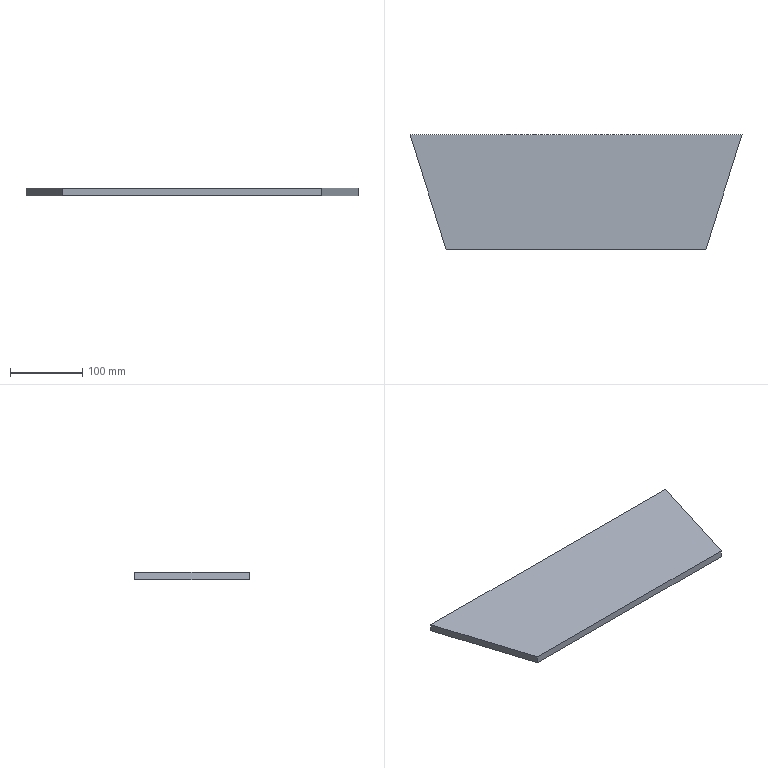Part | STEP file | 04-Vertical plate | 1 solid | 6 faces | box 460 x 159 x 10 mm | volume 651900 mm3 | plane 6
STEP:
#1=CARTESIAN_POINT('',(0.,0.,0.));
#2=DIRECTION('',(0.,0.,1.));
#3=DIRECTION('',(1.,0.,0.));
#4=AXIS2_PLACEMENT_3D('',#1,#2,#3);
#5=CARTESIAN_POINT('',(460.,0.,0.));
#6=VERTEX_POINT('',#5);
#7=CARTESIAN_POINT('',(0.,0.,0.));
#8=VERTEX_POINT('',#7);
#9=CARTESIAN_POINT('',(0.,0.,0.));
#10=DIRECTION('',(-1.,0.,0.));
#11=VECTOR('',#10,1.);
#12=LINE('',#9,#11);
#13=CARTESIAN_POINT('',(0.,0.,10.));
#14=DIRECTION('',(0.,-1.,0.));
#15=DIRECTION('',(0.,0.,-1.));
#16=AXIS2_PLACEMENT_3D('',#13,#14,#15);
#17=PLANE('',#16);
#18=CARTESIAN_POINT('',(10.,0.));
#19=DIRECTION('',(0.,-1.));
#20=VECTOR('',#19,1.);
#21=LINE('',#18,#20);
#22=(GEOMETRIC_REPRESENTATION_CONTEXT(2)PARAMETRIC_REPRESENTATION_CONTEXT()REPRESENTATION_CONTEXT('',''));
#23=DEFINITIONAL_REPRESENTATION('',(#21),#22);
#24=PCURVE('',#17,#23);
#25=CARTESIAN_POINT('',(0.,0.,0.));
#26=DIRECTION('',(0.,0.,-1.));
#27=DIRECTION('',(-1.,0.,0.));
#28=AXIS2_PLACEMENT_3D('',#25,#26,#27);
#29=PLANE('',#28);
#30=CARTESIAN_POINT('',(0.,0.));
#31=DIRECTION('',(1.,0.));
#32=VECTOR('',#31,1.);
#33=LINE('',#30,#32);
#34=(GEOMETRIC_REPRESENTATION_CONTEXT(2)PARAMETRIC_REPRESENTATION_CONTEXT()REPRESENTATION_CONTEXT('',''));
#35=DEFINITIONAL_REPRESENTATION('',(#33),#34);
#36=PCURVE('',#29,#35);
#37=SURFACE_CURVE('',#12,(#24,#36),.PCURVE_S1.);
#38=EDGE_CURVE('',#6,#8,#37,.T.);
#39=ORIENTED_EDGE('',*,*,#38,.T.);
#40=CARTESIAN_POINT('',(0.,0.,10.));
#41=VERTEX_POINT('',#40);
#42=CARTESIAN_POINT('',(0.,0.,10.));
#43=DIRECTION('',(0.,0.,-1.));
#44=VECTOR('',#43,1.);
#45=LINE('',#42,#44);
#46=CARTESIAN_POINT('',(0.,0.));
#47=DIRECTION('',(1.,0.));
#48=VECTOR('',#47,1.);
#49=LINE('',#46,#48);
#50=(GEOMETRIC_REPRESENTATION_CONTEXT(2)PARAMETRIC_REPRESENTATION_CONTEXT()REPRESENTATION_CONTEXT('',''));
#51=DEFINITIONAL_REPRESENTATION('',(#49),#50);
#52=PCURVE('',#17,#51);
#53=CARTESIAN_POINT('',(0.,0.,10.));
#54=DIRECTION('',(0.9539,0.3,0.));
#55=DIRECTION('',(-0.3,0.9539,0.));
#56=AXIS2_PLACEMENT_3D('',#53,#54,#55);
#57=PLANE('',#56);
#58=CARTESIAN_POINT('',(0.,0.));
#59=DIRECTION('',(0.,-1.));
#60=VECTOR('',#59,1.);
#61=LINE('',#58,#60);
#62=(GEOMETRIC_REPRESENTATION_CONTEXT(2)PARAMETRIC_REPRESENTATION_CONTEXT()REPRESENTATION_CONTEXT('',''));
#63=DEFINITIONAL_REPRESENTATION('',(#61),#62);
#64=PCURVE('',#57,#63);
#65=SURFACE_CURVE('',#45,(#52,#64),.PCURVE_S1.);
#66=EDGE_CURVE('',#41,#8,#65,.T.);
#67=ORIENTED_EDGE('',*,*,#66,.F.);
#68=CARTESIAN_POINT('',(460.,0.,10.));
#69=VERTEX_POINT('',#68);
#70=CARTESIAN_POINT('',(0.,0.,10.));
#71=DIRECTION('',(-1.,0.,0.));
#72=VECTOR('',#71,1.);
#73=LINE('',#70,#72);
#74=CARTESIAN_POINT('',(0.,0.));
#75=DIRECTION('',(0.,-1.));
#76=VECTOR('',#75,1.);
#77=LINE('',#74,#76);
#78=(GEOMETRIC_REPRESENTATION_CONTEXT(2)PARAMETRIC_REPRESENTATION_CONTEXT()REPRESENTATION_CONTEXT('',''));
#79=DEFINITIONAL_REPRESENTATION('',(#77),#78);
#80=PCURVE('',#17,#79);
#81=CARTESIAN_POINT('',(0.,0.,10.));
#82=DIRECTION('',(0.,0.,-1.));
#83=DIRECTION('',(-1.,0.,0.));
#84=AXIS2_PLACEMENT_3D('',#81,#82,#83);
#85=PLANE('',#84);
#86=CARTESIAN_POINT('',(0.,0.));
#87=DIRECTION('',(1.,0.));
#88=VECTOR('',#87,1.);
#89=LINE('',#86,#88);
#90=(GEOMETRIC_REPRESENTATION_CONTEXT(2)PARAMETRIC_REPRESENTATION_CONTEXT()REPRESENTATION_CONTEXT('',''));
#91=DEFINITIONAL_REPRESENTATION('',(#89),#90);
#92=PCURVE('',#85,#91);
#93=SURFACE_CURVE('',#73,(#80,#92),.PCURVE_S1.);
#94=EDGE_CURVE('',#69,#41,#93,.T.);
#95=ORIENTED_EDGE('',*,*,#94,.F.);
#96=CARTESIAN_POINT('',(460.,0.,10.));
#97=DIRECTION('',(0.,0.,-1.));
#98=VECTOR('',#97,1.);
#99=LINE('',#96,#98);
#100=CARTESIAN_POINT('',(0.,460.));
#101=DIRECTION('',(1.,0.));
#102=VECTOR('',#101,1.);
#103=LINE('',#100,#102);
#104=(GEOMETRIC_REPRESENTATION_CONTEXT(2)PARAMETRIC_REPRESENTATION_CONTEXT()REPRESENTATION_CONTEXT('',''));
#105=DEFINITIONAL_REPRESENTATION('',(#103),#104);
#106=PCURVE('',#17,#105);
#107=CARTESIAN_POINT('',(460.,0.,10.));
#108=DIRECTION('',(-0.9539,0.3,0.));
#109=DIRECTION('',(-0.3,-0.9539,0.));
#110=AXIS2_PLACEMENT_3D('',#107,#108,#109);
#111=PLANE('',#110);
#112=CARTESIAN_POINT('',(0.,0.));
#113=DIRECTION('',(0.,-1.));
#114=VECTOR('',#113,1.);
#115=LINE('',#112,#114);
#116=(GEOMETRIC_REPRESENTATION_CONTEXT(2)PARAMETRIC_REPRESENTATION_CONTEXT()REPRESENTATION_CONTEXT('',''));
#117=DEFINITIONAL_REPRESENTATION('',(#115),#116);
#118=PCURVE('',#111,#117);
#119=SURFACE_CURVE('',#99,(#106,#118),.PCURVE_S1.);
#120=EDGE_CURVE('',#69,#6,#119,.T.);
#121=ORIENTED_EDGE('',*,*,#120,.T.);
#122=EDGE_LOOP('',(#39,#67,#95,#121));
#123=FACE_BOUND('',#122,.T.);
#124=ADVANCED_FACE('',(#123),#17,.F.);
#125=CARTESIAN_POINT('',(50.,-159.,0.));
#126=VERTEX_POINT('',#125);
#127=CARTESIAN_POINT('',(0.,0.,0.));
#128=DIRECTION('',(0.3,-0.9539,0.));
#129=VECTOR('',#128,1.);
#130=LINE('',#127,#129);
#131=CARTESIAN_POINT('',(0.,-10.));
#132=DIRECTION('',(-1.,0.));
#133=VECTOR('',#132,1.);
#134=LINE('',#131,#133);
#135=(GEOMETRIC_REPRESENTATION_CONTEXT(2)PARAMETRIC_REPRESENTATION_CONTEXT()REPRESENTATION_CONTEXT('',''));
#136=DEFINITIONAL_REPRESENTATION('',(#134),#135);
#137=PCURVE('',#57,#136);
#138=CARTESIAN_POINT('',(0.,0.));
#139=DIRECTION('',(-0.3,-0.9539));
#140=VECTOR('',#139,1.);
#141=LINE('',#138,#140);
#142=(GEOMETRIC_REPRESENTATION_CONTEXT(2)PARAMETRIC_REPRESENTATION_CONTEXT()REPRESENTATION_CONTEXT('',''));
#143=DEFINITIONAL_REPRESENTATION('',(#141),#142);
#144=PCURVE('',#29,#143);
#145=SURFACE_CURVE('',#130,(#137,#144),.PCURVE_S1.);
#146=EDGE_CURVE('',#8,#126,#145,.T.);
#147=ORIENTED_EDGE('',*,*,#146,.T.);
#148=CARTESIAN_POINT('',(50.,-159.,10.));
#149=VERTEX_POINT('',#148);
#150=CARTESIAN_POINT('',(50.,-159.,10.));
#151=DIRECTION('',(0.,0.,-1.));
#152=VECTOR('',#151,1.);
#153=LINE('',#150,#152);
#154=CARTESIAN_POINT('',(-166.676,0.));
#155=DIRECTION('',(0.,-1.));
#156=VECTOR('',#155,1.);
#157=LINE('',#154,#156);
#158=(GEOMETRIC_REPRESENTATION_CONTEXT(2)PARAMETRIC_REPRESENTATION_CONTEXT()REPRESENTATION_CONTEXT('',''));
#159=DEFINITIONAL_REPRESENTATION('',(#157),#158);
#160=PCURVE('',#57,#159);
#161=CARTESIAN_POINT('',(50.,-159.,10.));
#162=DIRECTION('',(0.,1.,0.));
#163=DIRECTION('',(0.,0.,1.));
#164=AXIS2_PLACEMENT_3D('',#161,#162,#163);
#165=PLANE('',#164);
#166=CARTESIAN_POINT('',(0.,0.));
#167=DIRECTION('',(-1.,0.));
#168=VECTOR('',#167,1.);
#169=LINE('',#166,#168);
#170=(GEOMETRIC_REPRESENTATION_CONTEXT(2)PARAMETRIC_REPRESENTATION_CONTEXT()REPRESENTATION_CONTEXT('',''));
#171=DEFINITIONAL_REPRESENTATION('',(#169),#170);
#172=PCURVE('',#165,#171);
#173=SURFACE_CURVE('',#153,(#160,#172),.PCURVE_S1.);
#174=EDGE_CURVE('',#149,#126,#173,.T.);
#175=ORIENTED_EDGE('',*,*,#174,.F.);
#176=CARTESIAN_POINT('',(0.,0.,10.));
#177=DIRECTION('',(0.3,-0.9539,0.));
#178=VECTOR('',#177,1.);
#179=LINE('',#176,#178);
#180=CARTESIAN_POINT('',(0.,0.));
#181=DIRECTION('',(-1.,0.));
#182=VECTOR('',#181,1.);
#183=LINE('',#180,#182);
#184=(GEOMETRIC_REPRESENTATION_CONTEXT(2)PARAMETRIC_REPRESENTATION_CONTEXT()REPRESENTATION_CONTEXT('',''));
#185=DEFINITIONAL_REPRESENTATION('',(#183),#184);
#186=PCURVE('',#57,#185);
#187=CARTESIAN_POINT('',(0.,0.));
#188=DIRECTION('',(-0.3,-0.9539));
#189=VECTOR('',#188,1.);
#190=LINE('',#187,#189);
#191=(GEOMETRIC_REPRESENTATION_CONTEXT(2)PARAMETRIC_REPRESENTATION_CONTEXT()REPRESENTATION_CONTEXT('',''));
#192=DEFINITIONAL_REPRESENTATION('',(#190),#191);
#193=PCURVE('',#85,#192);
#194=SURFACE_CURVE('',#179,(#186,#193),.PCURVE_S1.);
#195=EDGE_CURVE('',#41,#149,#194,.T.);
#196=ORIENTED_EDGE('',*,*,#195,.F.);
#197=ORIENTED_EDGE('',*,*,#66,.T.);
#198=EDGE_LOOP('',(#147,#175,#196,#197));
#199=FACE_BOUND('',#198,.T.);
#200=ADVANCED_FACE('',(#199),#57,.F.);
#201=CARTESIAN_POINT('',(410.,-159.,0.));
#202=VERTEX_POINT('',#201);
#203=CARTESIAN_POINT('',(50.,-159.,0.));
#204=DIRECTION('',(1.,0.,0.));
#205=VECTOR('',#204,1.);
#206=LINE('',#203,#205);
#207=CARTESIAN_POINT('',(-10.,0.));
#208=DIRECTION('',(0.,1.));
#209=VECTOR('',#208,1.);
#210=LINE('',#207,#209);
#211=(GEOMETRIC_REPRESENTATION_CONTEXT(2)PARAMETRIC_REPRESENTATION_CONTEXT()REPRESENTATION_CONTEXT('',''));
#212=DEFINITIONAL_REPRESENTATION('',(#210),#211);
#213=PCURVE('',#165,#212);
#214=CARTESIAN_POINT('',(-50.,-159.));
#215=DIRECTION('',(-1.,0.));
#216=VECTOR('',#215,1.);
#217=LINE('',#214,#216);
#218=(GEOMETRIC_REPRESENTATION_CONTEXT(2)PARAMETRIC_REPRESENTATION_CONTEXT()REPRESENTATION_CONTEXT('',''));
#219=DEFINITIONAL_REPRESENTATION('',(#217),#218);
#220=PCURVE('',#29,#219);
#221=SURFACE_CURVE('',#206,(#213,#220),.PCURVE_S1.);
#222=EDGE_CURVE('',#126,#202,#221,.T.);
#223=ORIENTED_EDGE('',*,*,#222,.T.);
#224=CARTESIAN_POINT('',(410.,-159.,10.));
#225=VERTEX_POINT('',#224);
#226=CARTESIAN_POINT('',(410.,-159.,10.));
#227=DIRECTION('',(0.,0.,-1.));
#228=VECTOR('',#227,1.);
#229=LINE('',#226,#228);
#230=CARTESIAN_POINT('',(0.,360.));
#231=DIRECTION('',(-1.,0.));
#232=VECTOR('',#231,1.);
#233=LINE('',#230,#232);
#234=(GEOMETRIC_REPRESENTATION_CONTEXT(2)PARAMETRIC_REPRESENTATION_CONTEXT()REPRESENTATION_CONTEXT('',''));
#235=DEFINITIONAL_REPRESENTATION('',(#233),#234);
#236=PCURVE('',#165,#235);
#237=CARTESIAN_POINT('',(166.676,0.));
#238=DIRECTION('',(0.,-1.));
#239=VECTOR('',#238,1.);
#240=LINE('',#237,#239);
#241=(GEOMETRIC_REPRESENTATION_CONTEXT(2)PARAMETRIC_REPRESENTATION_CONTEXT()REPRESENTATION_CONTEXT('',''));
#242=DEFINITIONAL_REPRESENTATION('',(#240),#241);
#243=PCURVE('',#111,#242);
#244=SURFACE_CURVE('',#229,(#236,#243),.PCURVE_S1.);
#245=EDGE_CURVE('',#225,#202,#244,.T.);
#246=ORIENTED_EDGE('',*,*,#245,.F.);
#247=CARTESIAN_POINT('',(50.,-159.,10.));
#248=DIRECTION('',(1.,0.,0.));
#249=VECTOR('',#248,1.);
#250=LINE('',#247,#249);
#251=CARTESIAN_POINT('',(0.,0.));
#252=DIRECTION('',(0.,1.));
#253=VECTOR('',#252,1.);
#254=LINE('',#251,#253);
#255=(GEOMETRIC_REPRESENTATION_CONTEXT(2)PARAMETRIC_REPRESENTATION_CONTEXT()REPRESENTATION_CONTEXT('',''));
#256=DEFINITIONAL_REPRESENTATION('',(#254),#255);
#257=PCURVE('',#165,#256);
#258=CARTESIAN_POINT('',(-50.,-159.));
#259=DIRECTION('',(-1.,0.));
#260=VECTOR('',#259,1.);
#261=LINE('',#258,#260);
#262=(GEOMETRIC_REPRESENTATION_CONTEXT(2)PARAMETRIC_REPRESENTATION_CONTEXT()REPRESENTATION_CONTEXT('',''));
#263=DEFINITIONAL_REPRESENTATION('',(#261),#262);
#264=PCURVE('',#85,#263);
#265=SURFACE_CURVE('',#250,(#257,#264),.PCURVE_S1.);
#266=EDGE_CURVE('',#149,#225,#265,.T.);
#267=ORIENTED_EDGE('',*,*,#266,.F.);
#268=ORIENTED_EDGE('',*,*,#174,.T.);
#269=EDGE_LOOP('',(#223,#246,#267,#268));
#270=FACE_BOUND('',#269,.T.);
#271=ADVANCED_FACE('',(#270),#165,.F.);
#272=CARTESIAN_POINT('',(460.,0.,0.));
#273=DIRECTION('',(0.3,0.9539,0.));
#274=VECTOR('',#273,1.);
#275=LINE('',#272,#274);
#276=CARTESIAN_POINT('',(0.,-10.));
#277=DIRECTION('',(-1.,0.));
#278=VECTOR('',#277,1.);
#279=LINE('',#276,#278);
#280=(GEOMETRIC_REPRESENTATION_CONTEXT(2)PARAMETRIC_REPRESENTATION_CONTEXT()REPRESENTATION_CONTEXT('',''));
#281=DEFINITIONAL_REPRESENTATION('',(#279),#280);
#282=PCURVE('',#111,#281);
#283=CARTESIAN_POINT('',(-460.,0.));
#284=DIRECTION('',(-0.3,0.9539));
#285=VECTOR('',#284,1.);
#286=LINE('',#283,#285);
#287=(GEOMETRIC_REPRESENTATION_CONTEXT(2)PARAMETRIC_REPRESENTATION_CONTEXT()REPRESENTATION_CONTEXT('',''));
#288=DEFINITIONAL_REPRESENTATION('',(#286),#287);
#289=PCURVE('',#29,#288);
#290=SURFACE_CURVE('',#275,(#282,#289),.PCURVE_S1.);
#291=EDGE_CURVE('',#202,#6,#290,.T.);
#292=ORIENTED_EDGE('',*,*,#291,.T.);
#293=ORIENTED_EDGE('',*,*,#120,.F.);
#294=CARTESIAN_POINT('',(460.,0.,10.));
#295=DIRECTION('',(0.3,0.9539,0.));
#296=VECTOR('',#295,1.);
#297=LINE('',#294,#296);
#298=CARTESIAN_POINT('',(0.,0.));
#299=DIRECTION('',(-1.,0.));
#300=VECTOR('',#299,1.);
#301=LINE('',#298,#300);
#302=(GEOMETRIC_REPRESENTATION_CONTEXT(2)PARAMETRIC_REPRESENTATION_CONTEXT()REPRESENTATION_CONTEXT('',''));
#303=DEFINITIONAL_REPRESENTATION('',(#301),#302);
#304=PCURVE('',#111,#303);
#305=CARTESIAN_POINT('',(-460.,0.));
#306=DIRECTION('',(-0.3,0.9539));
#307=VECTOR('',#306,1.);
#308=LINE('',#305,#307);
#309=(GEOMETRIC_REPRESENTATION_CONTEXT(2)PARAMETRIC_REPRESENTATION_CONTEXT()REPRESENTATION_CONTEXT('',''));
#310=DEFINITIONAL_REPRESENTATION('',(#308),#309);
#311=PCURVE('',#85,#310);
#312=SURFACE_CURVE('',#297,(#304,#311),.PCURVE_S1.);
#313=EDGE_CURVE('',#225,#69,#312,.T.);
#314=ORIENTED_EDGE('',*,*,#313,.F.);
#315=ORIENTED_EDGE('',*,*,#245,.T.);
#316=EDGE_LOOP('',(#292,#293,#314,#315));
#317=FACE_BOUND('',#316,.T.);
#318=ADVANCED_FACE('',(#317),#111,.F.);
#319=ORIENTED_EDGE('',*,*,#94,.T.);
#320=ORIENTED_EDGE('',*,*,#195,.T.);
#321=ORIENTED_EDGE('',*,*,#266,.T.);
#322=ORIENTED_EDGE('',*,*,#313,.T.);
#323=EDGE_LOOP('',(#319,#320,#321,#322));
#324=FACE_BOUND('',#323,.T.);
#325=ADVANCED_FACE('',(#324),#85,.F.);
#326=ORIENTED_EDGE('',*,*,#38,.F.);
#327=ORIENTED_EDGE('',*,*,#291,.F.);
#328=ORIENTED_EDGE('',*,*,#222,.F.);
#329=ORIENTED_EDGE('',*,*,#146,.F.);
#330=EDGE_LOOP('',(#326,#327,#328,#329));
#331=FACE_BOUND('',#330,.T.);
#332=ADVANCED_FACE('',(#331),#29,.T.);
#333=CLOSED_SHELL('',(#124,#200,#271,#318,#325,#332));
#334=MANIFOLD_SOLID_BREP('',#333);
#335=(LENGTH_UNIT()NAMED_UNIT(*)SI_UNIT(.MILLI.,.METRE.));
#336=UNCERTAINTY_MEASURE_WITH_UNIT(LENGTH_MEASURE(0.0000001),#335,'','');
#337=(NAMED_UNIT(*)PLANE_ANGLE_UNIT()SI_UNIT($,.RADIAN.));
#338=(NAMED_UNIT(*)SI_UNIT($,.STERADIAN.)SOLID_ANGLE_UNIT());
#339=(GEOMETRIC_REPRESENTATION_CONTEXT(3)GLOBAL_UNCERTAINTY_ASSIGNED_CONTEXT((#336))GLOBAL_UNIT_ASSIGNED_CONTEXT((#335,#337,#338))REPRESENTATION_CONTEXT('',''));
#340=ADVANCED_BREP_SHAPE_REPRESENTATION('',(#4,#334),#339);